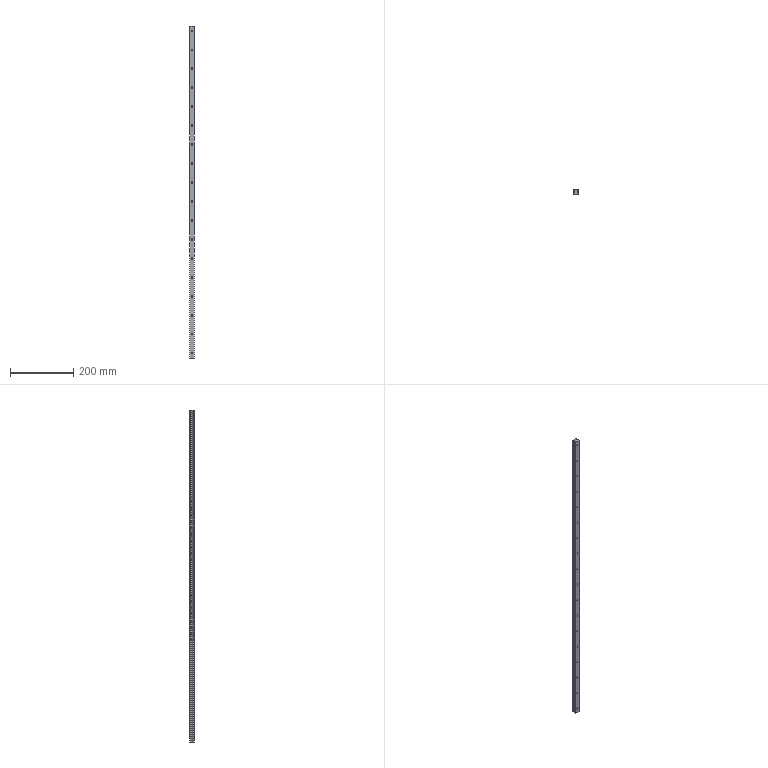Part | STEP file | HGR15-1050 | 1 solid | 126 faces | box 15 x 15 x 1050 mm | volume 193306 mm3 | cylinder 86 | plane 40 | commonest cylinder face diameters 4.5 x36 7.5 x36 0.8 x8 3.24 x4 2 x2